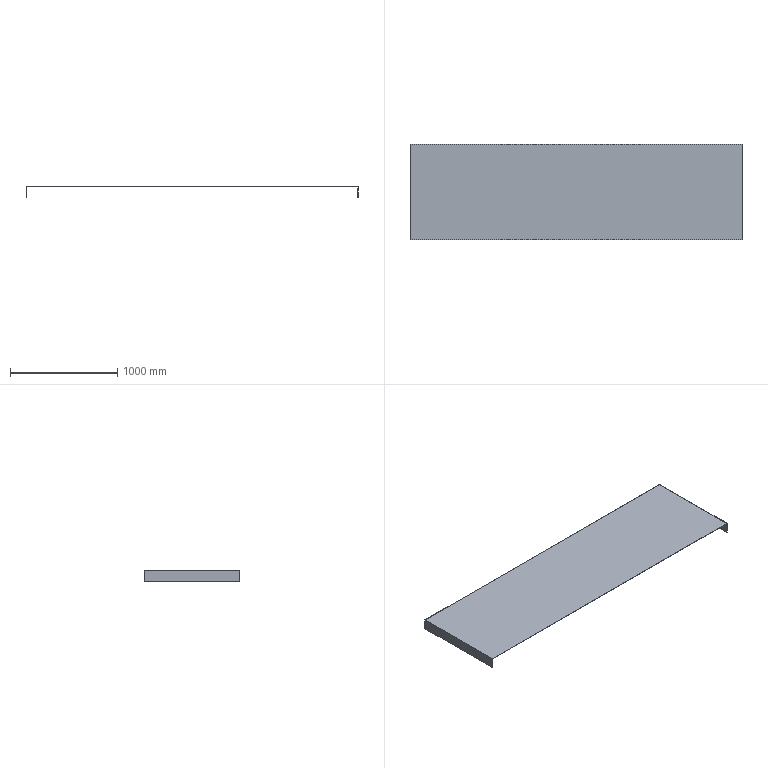Part | NX | features BREP 1 | 1 solid | 10 faces | box 3100 x 890 x 100 mm | volume 8794980 mm3 | plane 10
STEP:
#1=CARTESIAN_POINT('',(-1550.,445.,100.));
#2=VERTEX_POINT('',#1);
#3=CARTESIAN_POINT('',(-1550.,-445.,100.));
#4=VERTEX_POINT('',#3);
#5=CARTESIAN_POINT('',(-1550.,0.,100.));
#6=DIRECTION('',(0.,-1.,0.));
#7=VECTOR('',#6,1000.);
#8=LINE('',#5,#7);
#9=EDGE_CURVE('',#2,#4,#8,.T.);
#10=ORIENTED_EDGE('',*,*,#9,.T.);
#11=CARTESIAN_POINT('',(1550.,-445.,100.));
#12=VERTEX_POINT('',#11);
#13=CARTESIAN_POINT('',(0.,-445.,100.));
#14=DIRECTION('',(1.,0.,0.));
#15=VECTOR('',#14,1000.);
#16=LINE('',#13,#15);
#17=EDGE_CURVE('',#4,#12,#16,.T.);
#18=ORIENTED_EDGE('',*,*,#17,.T.);
#19=CARTESIAN_POINT('',(1550.,445.,100.));
#20=VERTEX_POINT('',#19);
#21=CARTESIAN_POINT('',(1550.,0.,100.));
#22=DIRECTION('',(0.,1.,0.));
#23=VECTOR('',#22,1000.);
#24=LINE('',#21,#23);
#25=EDGE_CURVE('',#12,#20,#24,.T.);
#26=ORIENTED_EDGE('',*,*,#25,.T.);
#27=CARTESIAN_POINT('',(0.,445.,100.));
#28=DIRECTION('',(-1.,0.,0.));
#29=VECTOR('',#28,1000.);
#30=LINE('',#27,#29);
#31=EDGE_CURVE('',#20,#2,#30,.T.);
#32=ORIENTED_EDGE('',*,*,#31,.T.);
#33=EDGE_LOOP('',(#10,#18,#26,#32));
#34=FACE_BOUND('',#33,.T.);
#35=CARTESIAN_POINT('',(0.,0.,100.));
#36=DIRECTION('',(0.,0.,1.));
#37=DIRECTION('',(1.,0.,0.));
#38=AXIS2_PLACEMENT_3D('',#35,#36,#37);
#39=PLANE('',#38);
#40=ADVANCED_FACE('',(#34),#39,.T.);
#41=CARTESIAN_POINT('',(-1550.,-445.,0.));
#42=VERTEX_POINT('',#41);
#43=CARTESIAN_POINT('',(-1547.,-445.,0.));
#44=VERTEX_POINT('',#43);
#45=CARTESIAN_POINT('',(1550.,-445.,0.));
#46=DIRECTION('',(1.,0.,0.));
#47=VECTOR('',#46,1000.);
#48=LINE('',#45,#47);
#49=EDGE_CURVE('',#42,#44,#48,.T.);
#50=ORIENTED_EDGE('',*,*,#49,.T.);
#51=CARTESIAN_POINT('',(-1547.,-445.,97.));
#52=VERTEX_POINT('',#51);
#53=CARTESIAN_POINT('',(-1547.,-445.,100.));
#54=DIRECTION('',(0.,0.,1.));
#55=VECTOR('',#54,1000.);
#56=LINE('',#53,#55);
#57=EDGE_CURVE('',#44,#52,#56,.T.);
#58=ORIENTED_EDGE('',*,*,#57,.T.);
#59=CARTESIAN_POINT('',(1547.,-445.,97.));
#60=VERTEX_POINT('',#59);
#61=CARTESIAN_POINT('',(1550.,-445.,97.));
#62=DIRECTION('',(1.,0.,0.));
#63=VECTOR('',#62,1000.);
#64=LINE('',#61,#63);
#65=EDGE_CURVE('',#52,#60,#64,.T.);
#66=ORIENTED_EDGE('',*,*,#65,.T.);
#67=CARTESIAN_POINT('',(1547.,-445.,0.));
#68=VERTEX_POINT('',#67);
#69=CARTESIAN_POINT('',(1547.,-445.,100.));
#70=DIRECTION('',(0.,0.,-1.));
#71=VECTOR('',#70,1000.);
#72=LINE('',#69,#71);
#73=EDGE_CURVE('',#60,#68,#72,.T.);
#74=ORIENTED_EDGE('',*,*,#73,.T.);
#75=CARTESIAN_POINT('',(1550.,-445.,0.));
#76=VERTEX_POINT('',#75);
#77=CARTESIAN_POINT('',(1550.,-445.,0.));
#78=DIRECTION('',(1.,0.,0.));
#79=VECTOR('',#78,1000.);
#80=LINE('',#77,#79);
#81=EDGE_CURVE('',#68,#76,#80,.T.);
#82=ORIENTED_EDGE('',*,*,#81,.T.);
#83=CARTESIAN_POINT('',(1550.,-445.,100.));
#84=DIRECTION('',(0.,0.,1.));
#85=VECTOR('',#84,1000.);
#86=LINE('',#83,#85);
#87=EDGE_CURVE('',#76,#12,#86,.T.);
#88=ORIENTED_EDGE('',*,*,#87,.T.);
#89=ORIENTED_EDGE('',*,*,#17,.F.);
#90=CARTESIAN_POINT('',(-1550.,-445.,100.));
#91=DIRECTION('',(0.,0.,-1.));
#92=VECTOR('',#91,1000.);
#93=LINE('',#90,#92);
#94=EDGE_CURVE('',#4,#42,#93,.T.);
#95=ORIENTED_EDGE('',*,*,#94,.T.);
#96=EDGE_LOOP('',(#50,#58,#66,#74,#82,#88,#89,#95));
#97=FACE_BOUND('',#96,.T.);
#98=CARTESIAN_POINT('',(1550.,-445.,100.));
#99=DIRECTION('',(0.,-1.,0.));
#100=DIRECTION('',(0.,0.,-1.));
#101=AXIS2_PLACEMENT_3D('',#98,#99,#100);
#102=PLANE('',#101);
#103=ADVANCED_FACE('',(#97),#102,.T.);
#104=ORIENTED_EDGE('',*,*,#9,.F.);
#105=CARTESIAN_POINT('',(-1550.,445.,0.));
#106=VERTEX_POINT('',#105);
#107=CARTESIAN_POINT('',(-1550.,445.,100.));
#108=DIRECTION('',(0.,0.,-1.));
#109=VECTOR('',#108,1000.);
#110=LINE('',#107,#109);
#111=EDGE_CURVE('',#2,#106,#110,.T.);
#112=ORIENTED_EDGE('',*,*,#111,.T.);
#113=CARTESIAN_POINT('',(-1550.,-445.,0.));
#114=DIRECTION('',(0.,-1.,0.));
#115=VECTOR('',#114,1000.);
#116=LINE('',#113,#115);
#117=EDGE_CURVE('',#106,#42,#116,.T.);
#118=ORIENTED_EDGE('',*,*,#117,.T.);
#119=ORIENTED_EDGE('',*,*,#94,.F.);
#120=EDGE_LOOP('',(#104,#112,#118,#119));
#121=FACE_BOUND('',#120,.T.);
#122=CARTESIAN_POINT('',(-1550.,-445.,100.));
#123=DIRECTION('',(-1.,0.,0.));
#124=DIRECTION('',(0.,0.,1.));
#125=AXIS2_PLACEMENT_3D('',#122,#123,#124);
#126=PLANE('',#125);
#127=ADVANCED_FACE('',(#121),#126,.T.);
#128=CARTESIAN_POINT('',(-1547.,445.,0.));
#129=VERTEX_POINT('',#128);
#130=CARTESIAN_POINT('',(-1547.,445.,97.));
#131=VERTEX_POINT('',#130);
#132=CARTESIAN_POINT('',(-1547.,445.,100.));
#133=DIRECTION('',(0.,0.,1.));
#134=VECTOR('',#133,1000.);
#135=LINE('',#132,#134);
#136=EDGE_CURVE('',#129,#131,#135,.T.);
#137=ORIENTED_EDGE('',*,*,#136,.F.);
#138=CARTESIAN_POINT('',(1550.,445.,0.));
#139=DIRECTION('',(1.,0.,0.));
#140=VECTOR('',#139,1000.);
#141=LINE('',#138,#140);
#142=EDGE_CURVE('',#106,#129,#141,.T.);
#143=ORIENTED_EDGE('',*,*,#142,.F.);
#144=ORIENTED_EDGE('',*,*,#111,.F.);
#145=ORIENTED_EDGE('',*,*,#31,.F.);
#146=CARTESIAN_POINT('',(1550.,445.,0.));
#147=VERTEX_POINT('',#146);
#148=CARTESIAN_POINT('',(1550.,445.,100.));
#149=DIRECTION('',(0.,0.,1.));
#150=VECTOR('',#149,1000.);
#151=LINE('',#148,#150);
#152=EDGE_CURVE('',#147,#20,#151,.T.);
#153=ORIENTED_EDGE('',*,*,#152,.F.);
#154=CARTESIAN_POINT('',(1547.,445.,0.));
#155=VERTEX_POINT('',#154);
#156=CARTESIAN_POINT('',(1550.,445.,0.));
#157=DIRECTION('',(1.,0.,0.));
#158=VECTOR('',#157,1000.);
#159=LINE('',#156,#158);
#160=EDGE_CURVE('',#155,#147,#159,.T.);
#161=ORIENTED_EDGE('',*,*,#160,.F.);
#162=CARTESIAN_POINT('',(1547.,445.,97.));
#163=VERTEX_POINT('',#162);
#164=CARTESIAN_POINT('',(1547.,445.,100.));
#165=DIRECTION('',(0.,0.,-1.));
#166=VECTOR('',#165,1000.);
#167=LINE('',#164,#166);
#168=EDGE_CURVE('',#163,#155,#167,.T.);
#169=ORIENTED_EDGE('',*,*,#168,.F.);
#170=CARTESIAN_POINT('',(1550.,445.,97.));
#171=DIRECTION('',(1.,0.,0.));
#172=VECTOR('',#171,1000.);
#173=LINE('',#170,#172);
#174=EDGE_CURVE('',#131,#163,#173,.T.);
#175=ORIENTED_EDGE('',*,*,#174,.F.);
#176=EDGE_LOOP('',(#137,#143,#144,#145,#153,#161,#169,#175));
#177=FACE_BOUND('',#176,.T.);
#178=CARTESIAN_POINT('',(1550.,445.,100.));
#179=DIRECTION('',(0.,-1.,0.));
#180=DIRECTION('',(0.,0.,-1.));
#181=AXIS2_PLACEMENT_3D('',#178,#179,#180);
#182=PLANE('',#181);
#183=ADVANCED_FACE('',(#177),#182,.F.);
#184=ORIENTED_EDGE('',*,*,#152,.T.);
#185=ORIENTED_EDGE('',*,*,#25,.F.);
#186=ORIENTED_EDGE('',*,*,#87,.F.);
#187=CARTESIAN_POINT('',(1550.,-445.,0.));
#188=DIRECTION('',(0.,-1.,0.));
#189=VECTOR('',#188,1000.);
#190=LINE('',#187,#189);
#191=EDGE_CURVE('',#147,#76,#190,.T.);
#192=ORIENTED_EDGE('',*,*,#191,.F.);
#193=EDGE_LOOP('',(#184,#185,#186,#192));
#194=FACE_BOUND('',#193,.T.);
#195=CARTESIAN_POINT('',(1550.,-445.,100.));
#196=DIRECTION('',(-1.,0.,0.));
#197=DIRECTION('',(0.,0.,1.));
#198=AXIS2_PLACEMENT_3D('',#195,#196,#197);
#199=PLANE('',#198);
#200=ADVANCED_FACE('',(#194),#199,.F.);
#201=ORIENTED_EDGE('',*,*,#136,.T.);
#202=CARTESIAN_POINT('',(-1547.,-445.,97.));
#203=DIRECTION('',(0.,1.,0.));
#204=VECTOR('',#203,1000.);
#205=LINE('',#202,#204);
#206=EDGE_CURVE('',#52,#131,#205,.T.);
#207=ORIENTED_EDGE('',*,*,#206,.F.);
#208=ORIENTED_EDGE('',*,*,#57,.F.);
#209=CARTESIAN_POINT('',(-1547.,-445.,0.));
#210=DIRECTION('',(0.,-1.,0.));
#211=VECTOR('',#210,1000.);
#212=LINE('',#209,#211);
#213=EDGE_CURVE('',#129,#44,#212,.T.);
#214=ORIENTED_EDGE('',*,*,#213,.F.);
#215=EDGE_LOOP('',(#201,#207,#208,#214));
#216=FACE_BOUND('',#215,.T.);
#217=CARTESIAN_POINT('',(-1547.,-445.,100.));
#218=DIRECTION('',(-1.,0.,0.));
#219=DIRECTION('',(0.,0.,1.));
#220=AXIS2_PLACEMENT_3D('',#217,#218,#219);
#221=PLANE('',#220);
#222=ADVANCED_FACE('',(#216),#221,.F.);
#223=ORIENTED_EDGE('',*,*,#49,.F.);
#224=ORIENTED_EDGE('',*,*,#117,.F.);
#225=ORIENTED_EDGE('',*,*,#142,.T.);
#226=ORIENTED_EDGE('',*,*,#213,.T.);
#227=EDGE_LOOP('',(#223,#224,#225,#226));
#228=FACE_BOUND('',#227,.T.);
#229=CARTESIAN_POINT('',(0.,0.,0.));
#230=DIRECTION('',(0.,0.,1.));
#231=DIRECTION('',(1.,0.,0.));
#232=AXIS2_PLACEMENT_3D('',#229,#230,#231);
#233=PLANE('',#232);
#234=ADVANCED_FACE('',(#228),#233,.F.);
#235=CARTESIAN_POINT('',(1547.,0.,0.));
#236=DIRECTION('',(0.,-1.,0.));
#237=VECTOR('',#236,1000.);
#238=LINE('',#235,#237);
#239=EDGE_CURVE('',#155,#68,#238,.T.);
#240=ORIENTED_EDGE('',*,*,#239,.F.);
#241=ORIENTED_EDGE('',*,*,#160,.T.);
#242=ORIENTED_EDGE('',*,*,#191,.T.);
#243=ORIENTED_EDGE('',*,*,#81,.F.);
#244=EDGE_LOOP('',(#240,#241,#242,#243));
#245=FACE_BOUND('',#244,.T.);
#246=CARTESIAN_POINT('',(0.,0.,0.));
#247=DIRECTION('',(0.,0.,1.));
#248=DIRECTION('',(1.,0.,0.));
#249=AXIS2_PLACEMENT_3D('',#246,#247,#248);
#250=PLANE('',#249);
#251=ADVANCED_FACE('',(#245),#250,.F.);
#252=CARTESIAN_POINT('',(1547.,-445.,97.));
#253=DIRECTION('',(0.,1.,0.));
#254=VECTOR('',#253,1000.);
#255=LINE('',#252,#254);
#256=EDGE_CURVE('',#60,#163,#255,.T.);
#257=ORIENTED_EDGE('',*,*,#256,.T.);
#258=ORIENTED_EDGE('',*,*,#168,.T.);
#259=ORIENTED_EDGE('',*,*,#239,.T.);
#260=ORIENTED_EDGE('',*,*,#73,.F.);
#261=EDGE_LOOP('',(#257,#258,#259,#260));
#262=FACE_BOUND('',#261,.T.);
#263=CARTESIAN_POINT('',(1547.,-445.,100.));
#264=DIRECTION('',(-1.,0.,0.));
#265=DIRECTION('',(0.,0.,1.));
#266=AXIS2_PLACEMENT_3D('',#263,#264,#265);
#267=PLANE('',#266);
#268=ADVANCED_FACE('',(#262),#267,.T.);
#269=ORIENTED_EDGE('',*,*,#65,.F.);
#270=ORIENTED_EDGE('',*,*,#206,.T.);
#271=ORIENTED_EDGE('',*,*,#174,.T.);
#272=ORIENTED_EDGE('',*,*,#256,.F.);
#273=EDGE_LOOP('',(#269,#270,#271,#272));
#274=FACE_BOUND('',#273,.T.);
#275=CARTESIAN_POINT('',(0.,0.,97.));
#276=DIRECTION('',(0.,0.,1.));
#277=DIRECTION('',(1.,0.,0.));
#278=AXIS2_PLACEMENT_3D('',#275,#276,#277);
#279=PLANE('',#278);
#280=ADVANCED_FACE('',(#274),#279,.F.);
#281=CLOSED_SHELL('',(#40,#103,#127,#183,#200,#222,#234,#251,#268,#280));
#282=MANIFOLD_SOLID_BREP('',#281);
#283=(LENGTH_UNIT()NAMED_UNIT(*)SI_UNIT(.MILLI.,.METRE.));
#284=UNCERTAINTY_MEASURE_WITH_UNIT(LENGTH_MEASURE(0.00001),#283,'','');
#285=(NAMED_UNIT(*)PLANE_ANGLE_UNIT()SI_UNIT($,.RADIAN.));
#286=(NAMED_UNIT(*)SI_UNIT($,.STERADIAN.)SOLID_ANGLE_UNIT());
#287=(GEOMETRIC_REPRESENTATION_CONTEXT(3)GLOBAL_UNCERTAINTY_ASSIGNED_CONTEXT((#284))GLOBAL_UNIT_ASSIGNED_CONTEXT((#283,#285,#286))REPRESENTATION_CONTEXT('',''));
#288=ADVANCED_BREP_SHAPE_REPRESENTATION('',(#282),#287);